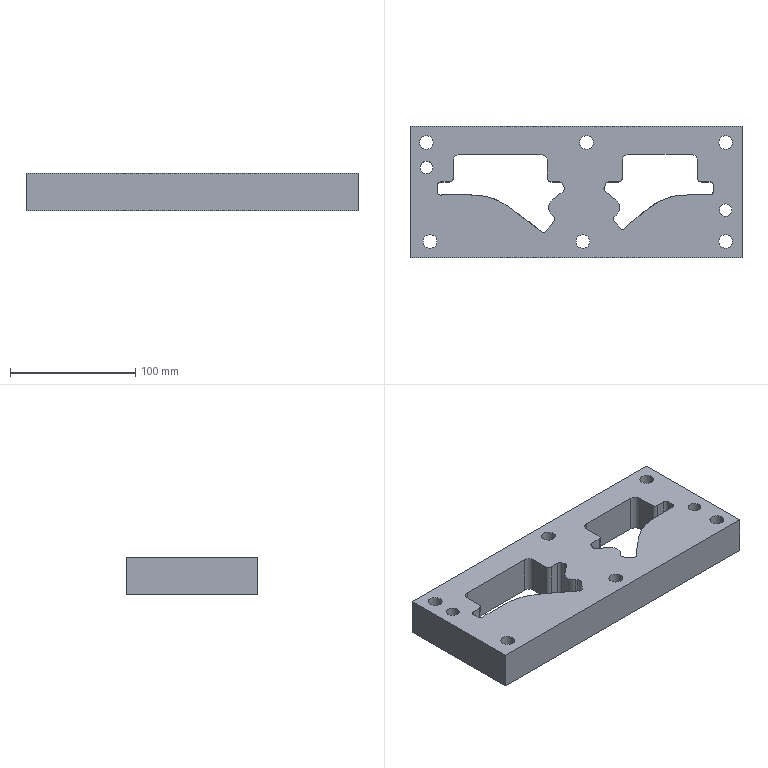Part | STEP file | 201_id730_x_t | 1 solid | 84 faces | box 265 x 105 x 30 mm | volume 611184 mm3 | cylinder 43 | plane 35 | other 6 | commonest cylinder face diameters 5 x13 11 x8 6 x6 10 x6 17 x6 16 x2